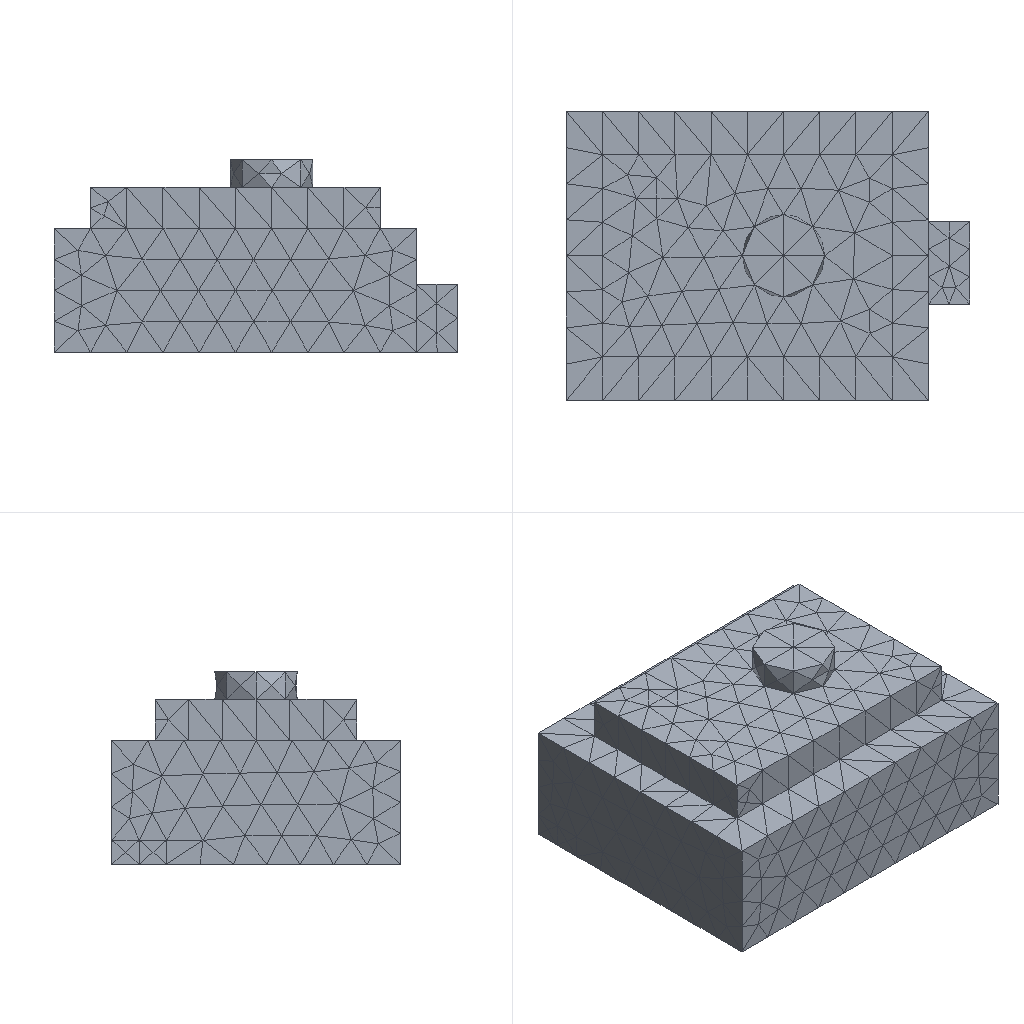Simulation study | ansys mapdl
Set-up summary:
category,name,step,type,value,unit,region
solver,ansys_mapdl
units,mm-N-s-tonne (MPa),,inferred,E=210000 density=
analysis,model,,static
mesh,nodes,,,5059
mesh,elements,,,3048
element_type,SOLID187,,,3048
material,mat 1,,E,210000
material,mat 1,,nu,0.3
load,,model,body load temp,,,all
load,,model,force,"1000 [dir=(0, 0, -1) n=367]",,node list
bc,,model,fixed,"[dofs=UX,UY,UZ n=5680]",,node list
Ansys APDL input file, long lists of numbers shortened:
/COM,ANSYS RELEASE 2026 R1           BUILD 26.1      UP20260202       09:08:47
/PREP7
/NOPR
/TITLE,2
ANTYPE, 0
*IF,_CDRDOFF,EQ,1,THEN     !if solid model was read in
_CDRDOFF=             !reset flag, numoffs already performed
*ELSE              !offset database for the following FE model
NUMOFF,NODE,     5059
NUMOFF,ELEM,     3048
NUMOFF,MAT ,        1
NUMOFF,TYPE,        1
*ENDIF
*SET,_RETURN ,  0.
*SET,_STATUS ,  0.
*SET,_UIQR   ,  367.
*SET,__FLOATPARAMETER__,  5059.
DOF,DELETE
ETBLOCK,        1,        1
(2i9,19a9)
        1      187        0        0        0        0        0        0        0        0        0        0        0        0        0        0        0        0        0        0        0
       -1
NBLOCK,6,SOLID,      5059,      5059
(3i9,6e21.13e3)
        1        0        0-3.6700000000000E+001 4.2000000000000E+001 7.0000000000000E+000
! (5058 more lines like these left out)
N,UNBL,LOC,       -1,
EBLOCK,19,SOLID,      3048,      3048
(19i10)
         1         1         1         1         0         0         0         0        10         0         1      1891      1892       227       516      2187      2188      2189      2190
! (6095 more lines like these left out)
        -1
MPTEMP,UNBL, 1, 1,  0.    ,
MPDATA,UNBL, 1,EX  ,       1, 1,  210000.000    ,
MPTEMP,UNBL, 1, 1,  0.    ,
MPDATA,UNBL, 1,NUXY,       1, 1, 0.3    ,
MPTEMP,UNBL, 1, 1,  0.    ,
MPDATA,UNBL, 1,PRXY,       1, 1, 0.3    ,
EXTOPT,ATTR,      0,      0,      0
EXTOPT,ESIZE,  0,  0.
EXTOPT,ACLEAR,      0
TREF,  0.
IRLF,  0
BFUNIF,TEMP,_TINY
ACEL,  0.    ,  0.    ,  0.
OMEGA,  0.    ,  0.    ,  0.
DOMEGA,  0.    ,  0.    ,  0.
CGLOC,  0.    ,  0.    ,  0.
CGOMEGA,  0.    ,  0.    ,  0.
DCGOMG,  0.    ,  0.    ,  0.
KUSE,     0
TIME,  0.
ALPHAD,  0.
BETAD,  0.
DMPRAT,  0.
DMPSTR,  0.
CRPLIM, 0.1    ,   0
CRPLIM,  0.    ,   1
NCNV,     0, 1.000000000E+12,     0,  0.    ,  0.
NEQIT,     0
ERESX,DEFA
DBLOCK,      5680
(i9,a6,2(pg16.9))
        1  UX    0.00000000      0.00000000
! (5679 more lines like these left out)
       -1
FBLOCK,       367
(i9,a6,2(pg16.9))
      584  FZ   -2.72479564      0.00000000
! (366 more lines like these left out)
       -1
/GO
FINISH
Results summary:
result,analysis_type_db,,,static,unstated
result,n_sets,,,1,unstated
result,load_steps[0].set,load_step=1,,1,unstated
result,load_steps[0].substep,load_step=1,,1,unstated
result,load_steps[0].time,load_step=1,,1,unstated
result,load_steps[0].freq,load_step=1,,1,unstated
result,load_steps[0].max_usum,load_step=1,,8.96395e-05,unstated
result,load_steps[0].max_seqv,load_step=1,,0.9993,unstated
result,load_steps[0].reaction_sum.FX,load_step=1,,-6.33937e-13,unstated
result,load_steps[0].reaction_sum.FY,load_step=1,,1.09956e-11,unstated
result,load_steps[0].reaction_sum.FZ,load_step=1,,1000,unstated
result,load_steps[0].reaction_sum.MX,load_step=1,,0,unstated
result,load_steps[0].reaction_sum.MY,load_step=1,,0,unstated
result,load_steps[0].reaction_sum.MZ,load_step=1,,0,unstated
result,convergence,,,results present for all listed sets,unstated